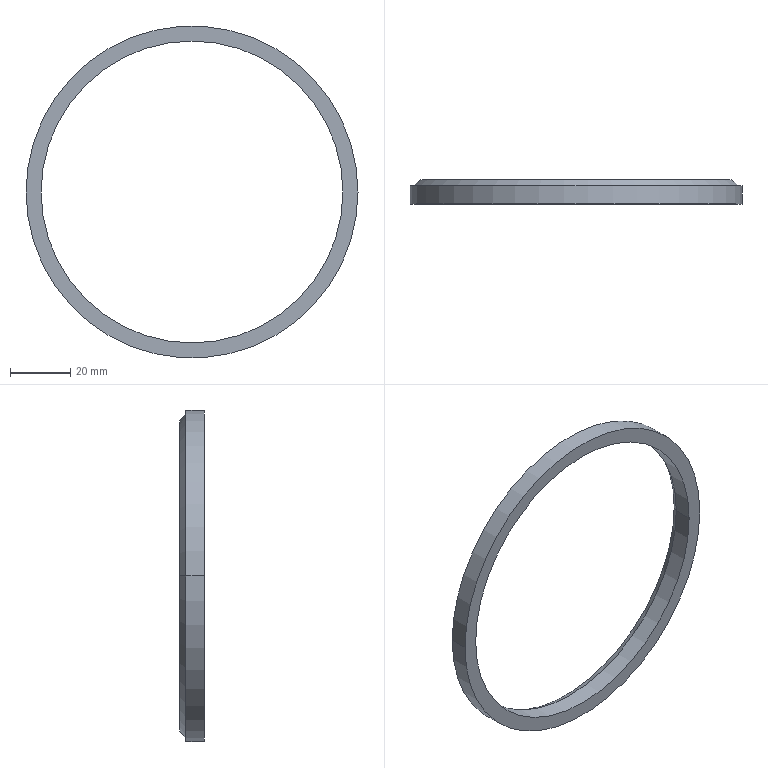Part | SolidWorks | features Revolution 1 | 1 solid | 11 faces | box 110 x 8 x 110 mm | volume 11358 mm3 | cone 4 | cylinder 4 | plane 3 | commonest cylinder face diameters 100 x2 110 x2
STEP:
#1=CARTESIAN_POINT('',(-50.,6.,0.));
#2=VERTEX_POINT('',#1);
#3=CARTESIAN_POINT('',(50.,6.,0.));
#4=VERTEX_POINT('',#3);
#5=CARTESIAN_POINT('',(0.,6.,0.));
#6=DIRECTION('',(0.,-1.,0.));
#7=DIRECTION('',(1.,0.,0.));
#8=AXIS2_PLACEMENT_3D('',#5,#6,#7);
#9=CIRCLE('',#8,50.);
#10=EDGE_CURVE('',#2,#4,#9,.T.);
#11=ORIENTED_EDGE('',*,*,#10,.T.);
#12=CARTESIAN_POINT('',(51.,8.,0.));
#13=VERTEX_POINT('',#12);
#14=CARTESIAN_POINT('',(51.,8.,0.));
#15=DIRECTION('',(0.4472,0.8944,0.));
#16=VECTOR('',#15,1000.);
#17=LINE('',#14,#16);
#18=EDGE_CURVE('',#4,#13,#17,.T.);
#19=ORIENTED_EDGE('',*,*,#18,.T.);
#20=CARTESIAN_POINT('',(-51.,8.,0.));
#21=VERTEX_POINT('',#20);
#22=CARTESIAN_POINT('',(0.,8.,0.));
#23=DIRECTION('',(0.,-1.,0.));
#24=DIRECTION('',(1.,0.,0.));
#25=AXIS2_PLACEMENT_3D('',#22,#23,#24);
#26=CIRCLE('',#25,51.);
#27=EDGE_CURVE('',#21,#13,#26,.T.);
#28=ORIENTED_EDGE('',*,*,#27,.F.);
#29=CARTESIAN_POINT('',(-51.,8.,0.));
#30=DIRECTION('',(-0.4472,0.8944,0.));
#31=VECTOR('',#30,1000.);
#32=LINE('',#29,#31);
#33=EDGE_CURVE('',#2,#21,#32,.T.);
#34=ORIENTED_EDGE('',*,*,#33,.F.);
#35=EDGE_LOOP('',(#11,#19,#28,#34));
#36=FACE_OUTER_BOUND('',#35,.T.);
#37=CARTESIAN_POINT('',(0.,8.,0.));
#38=DIRECTION('',(0.,1.,0.));
#39=DIRECTION('',(-1.,0.,0.));
#40=AXIS2_PLACEMENT_3D('',#37,#38,#39);
#41=CONICAL_SURFACE('',#40,51.,0.4636);
#42=ADVANCED_FACE('',(#36),#41,.F.);
#43=CARTESIAN_POINT('',(51.5,8.,0.));
#44=VERTEX_POINT('',#43);
#45=CARTESIAN_POINT('',(-51.5,8.,0.));
#46=VERTEX_POINT('',#45);
#47=CARTESIAN_POINT('',(0.,8.,0.));
#48=DIRECTION('',(0.,-1.,0.));
#49=DIRECTION('',(1.,0.,0.));
#50=AXIS2_PLACEMENT_3D('',#47,#48,#49);
#51=CIRCLE('',#50,51.5);
#52=EDGE_CURVE('',#44,#46,#51,.T.);
#53=ORIENTED_EDGE('',*,*,#52,.T.);
#54=CARTESIAN_POINT('',(-54.,6.,0.));
#55=VERTEX_POINT('',#54);
#56=CARTESIAN_POINT('',(-54.,6.,0.));
#57=DIRECTION('',(-0.7809,-0.6247,0.));
#58=VECTOR('',#57,1000.);
#59=LINE('',#56,#58);
#60=EDGE_CURVE('',#46,#55,#59,.T.);
#61=ORIENTED_EDGE('',*,*,#60,.T.);
#62=CARTESIAN_POINT('',(54.,6.,0.));
#63=VERTEX_POINT('',#62);
#64=CARTESIAN_POINT('',(0.,6.,0.));
#65=DIRECTION('',(0.,-1.,0.));
#66=DIRECTION('',(1.,0.,0.));
#67=AXIS2_PLACEMENT_3D('',#64,#65,#66);
#68=CIRCLE('',#67,54.);
#69=EDGE_CURVE('',#63,#55,#68,.T.);
#70=ORIENTED_EDGE('',*,*,#69,.F.);
#71=CARTESIAN_POINT('',(54.,6.,0.));
#72=DIRECTION('',(0.7809,-0.6247,0.));
#73=VECTOR('',#72,1000.);
#74=LINE('',#71,#73);
#75=EDGE_CURVE('',#44,#63,#74,.T.);
#76=ORIENTED_EDGE('',*,*,#75,.F.);
#77=EDGE_LOOP('',(#53,#61,#70,#76));
#78=FACE_OUTER_BOUND('',#77,.T.);
#79=CARTESIAN_POINT('',(0.,6.,0.));
#80=DIRECTION('',(0.,-1.,0.));
#81=DIRECTION('',(1.,0.,0.));
#82=AXIS2_PLACEMENT_3D('',#79,#80,#81);
#83=CONICAL_SURFACE('',#82,54.,0.8961);
#84=ADVANCED_FACE('',(#78),#83,.T.);
#85=CARTESIAN_POINT('',(55.,6.,0.));
#86=VERTEX_POINT('',#85);
#87=CARTESIAN_POINT('',(-55.,6.,0.));
#88=VERTEX_POINT('',#87);
#89=CARTESIAN_POINT('',(0.,6.,0.));
#90=DIRECTION('',(0.,-1.,0.));
#91=DIRECTION('',(1.,0.,0.));
#92=AXIS2_PLACEMENT_3D('',#89,#90,#91);
#93=CIRCLE('',#92,55.);
#94=EDGE_CURVE('',#86,#88,#93,.T.);
#95=ORIENTED_EDGE('',*,*,#94,.T.);
#96=CARTESIAN_POINT('',(-55.,0.,0.));
#97=VERTEX_POINT('',#96);
#98=CARTESIAN_POINT('',(-55.,-1000.,0.));
#99=DIRECTION('',(0.,-1.,0.));
#100=VECTOR('',#99,1000.);
#101=LINE('',#98,#100);
#102=EDGE_CURVE('',#88,#97,#101,.T.);
#103=ORIENTED_EDGE('',*,*,#102,.T.);
#104=CARTESIAN_POINT('',(55.,0.,0.));
#105=VERTEX_POINT('',#104);
#106=CARTESIAN_POINT('',(0.,0.,0.));
#107=DIRECTION('',(0.,-1.,0.));
#108=DIRECTION('',(1.,0.,0.));
#109=AXIS2_PLACEMENT_3D('',#106,#107,#108);
#110=CIRCLE('',#109,55.);
#111=EDGE_CURVE('',#105,#97,#110,.T.);
#112=ORIENTED_EDGE('',*,*,#111,.F.);
#113=CARTESIAN_POINT('',(55.,-1000.,0.));
#114=DIRECTION('',(0.,-1.,0.));
#115=VECTOR('',#114,1000.);
#116=LINE('',#113,#115);
#117=EDGE_CURVE('',#86,#105,#116,.T.);
#118=ORIENTED_EDGE('',*,*,#117,.F.);
#119=EDGE_LOOP('',(#95,#103,#112,#118));
#120=FACE_OUTER_BOUND('',#119,.T.);
#121=CARTESIAN_POINT('',(0.,-1000.,0.));
#122=DIRECTION('',(0.,-1.,0.));
#123=DIRECTION('',(1.,0.,0.));
#124=AXIS2_PLACEMENT_3D('',#121,#122,#123);
#125=CYLINDRICAL_SURFACE('',#124,55.);
#126=ADVANCED_FACE('',(#120),#125,.T.);
#127=ORIENTED_EDGE('',*,*,#10,.F.);
#128=CARTESIAN_POINT('',(-50.,0.,0.));
#129=VERTEX_POINT('',#128);
#130=CARTESIAN_POINT('',(-50.,-1000.,0.));
#131=DIRECTION('',(0.,-1.,0.));
#132=VECTOR('',#131,1000.);
#133=LINE('',#130,#132);
#134=EDGE_CURVE('',#2,#129,#133,.T.);
#135=ORIENTED_EDGE('',*,*,#134,.T.);
#136=CARTESIAN_POINT('',(50.,0.,0.));
#137=VERTEX_POINT('',#136);
#138=CARTESIAN_POINT('',(0.,0.,0.));
#139=DIRECTION('',(0.,-1.,0.));
#140=DIRECTION('',(1.,0.,0.));
#141=AXIS2_PLACEMENT_3D('',#138,#139,#140);
#142=CIRCLE('',#141,50.);
#143=EDGE_CURVE('',#129,#137,#142,.T.);
#144=ORIENTED_EDGE('',*,*,#143,.T.);
#145=CARTESIAN_POINT('',(50.,-1000.,0.));
#146=DIRECTION('',(0.,-1.,0.));
#147=VECTOR('',#146,1000.);
#148=LINE('',#145,#147);
#149=EDGE_CURVE('',#4,#137,#148,.T.);
#150=ORIENTED_EDGE('',*,*,#149,.F.);
#151=EDGE_LOOP('',(#127,#135,#144,#150));
#152=FACE_OUTER_BOUND('',#151,.T.);
#153=CARTESIAN_POINT('',(0.,-1000.,0.));
#154=DIRECTION('',(0.,-1.,0.));
#155=DIRECTION('',(1.,0.,0.));
#156=AXIS2_PLACEMENT_3D('',#153,#154,#155);
#157=CYLINDRICAL_SURFACE('',#156,50.);
#158=ADVANCED_FACE('',(#152),#157,.F.);
#159=ORIENTED_EDGE('',*,*,#134,.F.);
#160=CARTESIAN_POINT('',(0.,6.,0.));
#161=DIRECTION('',(0.,-1.,0.));
#162=DIRECTION('',(1.,0.,0.));
#163=AXIS2_PLACEMENT_3D('',#160,#161,#162);
#164=CIRCLE('',#163,50.);
#165=EDGE_CURVE('',#4,#2,#164,.T.);
#166=ORIENTED_EDGE('',*,*,#165,.F.);
#167=ORIENTED_EDGE('',*,*,#149,.T.);
#168=CARTESIAN_POINT('',(0.,0.,0.));
#169=DIRECTION('',(0.,-1.,0.));
#170=DIRECTION('',(1.,0.,0.));
#171=AXIS2_PLACEMENT_3D('',#168,#169,#170);
#172=CIRCLE('',#171,50.);
#173=EDGE_CURVE('',#137,#129,#172,.T.);
#174=ORIENTED_EDGE('',*,*,#173,.T.);
#175=EDGE_LOOP('',(#159,#166,#167,#174));
#176=FACE_OUTER_BOUND('',#175,.T.);
#177=CARTESIAN_POINT('',(0.,-1000.,0.));
#178=DIRECTION('',(0.,-1.,0.));
#179=DIRECTION('',(1.,0.,0.));
#180=AXIS2_PLACEMENT_3D('',#177,#178,#179);
#181=CYLINDRICAL_SURFACE('',#180,50.);
#182=ADVANCED_FACE('',(#176),#181,.F.);
#183=ORIENTED_EDGE('',*,*,#111,.T.);
#184=CARTESIAN_POINT('',(0.,0.,0.));
#185=DIRECTION('',(0.,-1.,0.));
#186=DIRECTION('',(1.,0.,0.));
#187=AXIS2_PLACEMENT_3D('',#184,#185,#186);
#188=CIRCLE('',#187,55.);
#189=EDGE_CURVE('',#97,#105,#188,.T.);
#190=ORIENTED_EDGE('',*,*,#189,.T.);
#191=EDGE_LOOP('',(#183,#190));
#192=FACE_OUTER_BOUND('',#191,.T.);
#193=ORIENTED_EDGE('',*,*,#173,.F.);
#194=ORIENTED_EDGE('',*,*,#143,.F.);
#195=EDGE_LOOP('',(#193,#194));
#196=FACE_BOUND('',#195,.T.);
#197=CARTESIAN_POINT('',(50.,0.,0.));
#198=DIRECTION('',(0.,-1.,0.));
#199=DIRECTION('',(1.,0.,0.));
#200=AXIS2_PLACEMENT_3D('',#197,#198,#199);
#201=PLANE('',#200);
#202=ADVANCED_FACE('',(#192,#196),#201,.T.);
#203=ORIENTED_EDGE('',*,*,#102,.F.);
#204=CARTESIAN_POINT('',(0.,6.,0.));
#205=DIRECTION('',(0.,-1.,0.));
#206=DIRECTION('',(1.,0.,0.));
#207=AXIS2_PLACEMENT_3D('',#204,#205,#206);
#208=CIRCLE('',#207,55.);
#209=EDGE_CURVE('',#88,#86,#208,.T.);
#210=ORIENTED_EDGE('',*,*,#209,.T.);
#211=ORIENTED_EDGE('',*,*,#117,.T.);
#212=ORIENTED_EDGE('',*,*,#189,.F.);
#213=EDGE_LOOP('',(#203,#210,#211,#212));
#214=FACE_OUTER_BOUND('',#213,.T.);
#215=CARTESIAN_POINT('',(0.,-1000.,0.));
#216=DIRECTION('',(0.,-1.,0.));
#217=DIRECTION('',(1.,0.,0.));
#218=AXIS2_PLACEMENT_3D('',#215,#216,#217);
#219=CYLINDRICAL_SURFACE('',#218,55.);
#220=ADVANCED_FACE('',(#214),#219,.T.);
#221=ORIENTED_EDGE('',*,*,#69,.T.);
#222=CARTESIAN_POINT('',(0.,6.,0.));
#223=DIRECTION('',(0.,-1.,0.));
#224=DIRECTION('',(1.,0.,0.));
#225=AXIS2_PLACEMENT_3D('',#222,#223,#224);
#226=CIRCLE('',#225,54.);
#227=EDGE_CURVE('',#55,#63,#226,.T.);
#228=ORIENTED_EDGE('',*,*,#227,.T.);
#229=EDGE_LOOP('',(#221,#228));
#230=FACE_BOUND('',#229,.T.);
#231=ORIENTED_EDGE('',*,*,#94,.F.);
#232=ORIENTED_EDGE('',*,*,#209,.F.);
#233=EDGE_LOOP('',(#231,#232));
#234=FACE_OUTER_BOUND('',#233,.T.);
#235=CARTESIAN_POINT('',(55.,6.,0.));
#236=DIRECTION('',(0.,1.,0.));
#237=DIRECTION('',(-1.,0.,0.));
#238=AXIS2_PLACEMENT_3D('',#235,#236,#237);
#239=PLANE('',#238);
#240=ADVANCED_FACE('',(#230,#234),#239,.T.);
#241=ORIENTED_EDGE('',*,*,#60,.F.);
#242=CARTESIAN_POINT('',(0.,8.,0.));
#243=DIRECTION('',(0.,-1.,0.));
#244=DIRECTION('',(1.,0.,0.));
#245=AXIS2_PLACEMENT_3D('',#242,#243,#244);
#246=CIRCLE('',#245,51.5);
#247=EDGE_CURVE('',#46,#44,#246,.T.);
#248=ORIENTED_EDGE('',*,*,#247,.T.);
#249=ORIENTED_EDGE('',*,*,#75,.T.);
#250=ORIENTED_EDGE('',*,*,#227,.F.);
#251=EDGE_LOOP('',(#241,#248,#249,#250));
#252=FACE_OUTER_BOUND('',#251,.T.);
#253=CARTESIAN_POINT('',(0.,6.,0.));
#254=DIRECTION('',(0.,-1.,0.));
#255=DIRECTION('',(1.,0.,0.));
#256=AXIS2_PLACEMENT_3D('',#253,#254,#255);
#257=CONICAL_SURFACE('',#256,54.,0.8961);
#258=ADVANCED_FACE('',(#252),#257,.T.);
#259=ORIENTED_EDGE('',*,*,#27,.T.);
#260=CARTESIAN_POINT('',(0.,8.,0.));
#261=DIRECTION('',(0.,-1.,0.));
#262=DIRECTION('',(1.,0.,0.));
#263=AXIS2_PLACEMENT_3D('',#260,#261,#262);
#264=CIRCLE('',#263,51.);
#265=EDGE_CURVE('',#13,#21,#264,.T.);
#266=ORIENTED_EDGE('',*,*,#265,.T.);
#267=EDGE_LOOP('',(#259,#266));
#268=FACE_BOUND('',#267,.T.);
#269=ORIENTED_EDGE('',*,*,#52,.F.);
#270=ORIENTED_EDGE('',*,*,#247,.F.);
#271=EDGE_LOOP('',(#269,#270));
#272=FACE_OUTER_BOUND('',#271,.T.);
#273=CARTESIAN_POINT('',(51.5,8.,0.));
#274=DIRECTION('',(0.,1.,0.));
#275=DIRECTION('',(-1.,0.,0.));
#276=AXIS2_PLACEMENT_3D('',#273,#274,#275);
#277=PLANE('',#276);
#278=ADVANCED_FACE('',(#268,#272),#277,.T.);
#279=ORIENTED_EDGE('',*,*,#18,.F.);
#280=ORIENTED_EDGE('',*,*,#165,.T.);
#281=ORIENTED_EDGE('',*,*,#33,.T.);
#282=ORIENTED_EDGE('',*,*,#265,.F.);
#283=EDGE_LOOP('',(#279,#280,#281,#282));
#284=FACE_OUTER_BOUND('',#283,.T.);
#285=CARTESIAN_POINT('',(0.,8.,0.));
#286=DIRECTION('',(0.,1.,0.));
#287=DIRECTION('',(-1.,0.,0.));
#288=AXIS2_PLACEMENT_3D('',#285,#286,#287);
#289=CONICAL_SURFACE('',#288,51.,0.4636);
#290=ADVANCED_FACE('',(#284),#289,.F.);
#291=CLOSED_SHELL('',(#42,#84,#126,#158,#182,#202,#220,#240,#258,#278,#290));
#292=MANIFOLD_SOLID_BREP('',#291);
#293=CARTESIAN_POINT('',(0.,0.,0.));
#294=DIRECTION('',(0.,0.,1.));
#295=DIRECTION('',(1.,0.,0.));
#296=AXIS2_PLACEMENT_3D('',#293,#294,#295);
#297=(LENGTH_UNIT()NAMED_UNIT(*)SI_UNIT(.MILLI.,.METRE.));
#298=UNCERTAINTY_MEASURE_WITH_UNIT(LENGTH_MEASURE(0.00001),#297,'','');
#299=(NAMED_UNIT(*)PLANE_ANGLE_UNIT()SI_UNIT($,.RADIAN.));
#300=(NAMED_UNIT(*)SI_UNIT($,.STERADIAN.)SOLID_ANGLE_UNIT());
#301=(GEOMETRIC_REPRESENTATION_CONTEXT(3)GLOBAL_UNCERTAINTY_ASSIGNED_CONTEXT((#298))GLOBAL_UNIT_ASSIGNED_CONTEXT((#297,#299,#300))REPRESENTATION_CONTEXT('',''));
#302=ADVANCED_BREP_SHAPE_REPRESENTATION('',(#292,#296),#301);